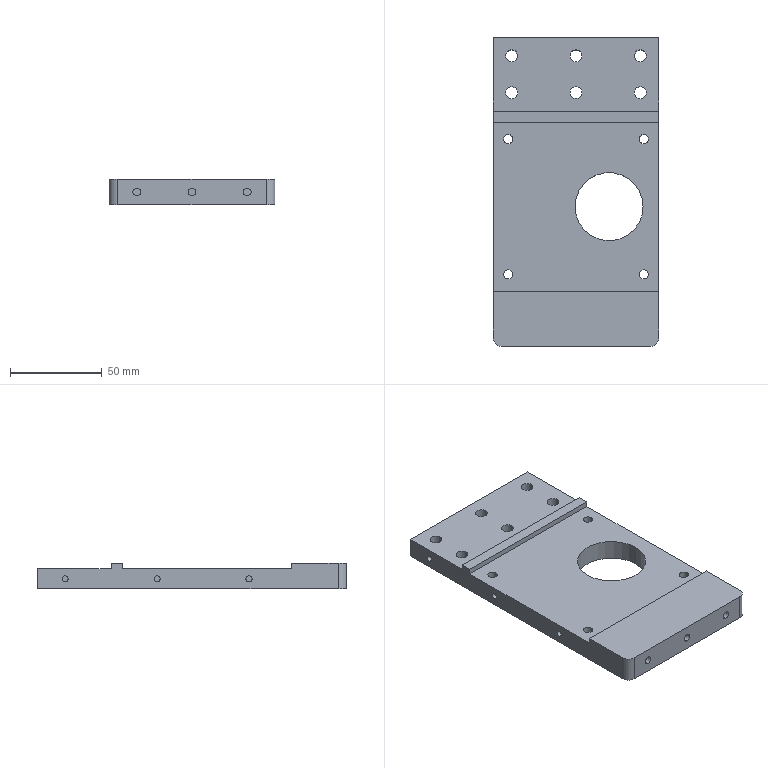Part | STEP file | 1 solid | 62 faces | box 90 x 168 x 14 mm | volume 160031 mm3 | cylinder 42 | plane 20 | commonest cylinder face diameters 3.3 x12 6.5 x12 5 x8 4.2 x6 9 x2 37 x2